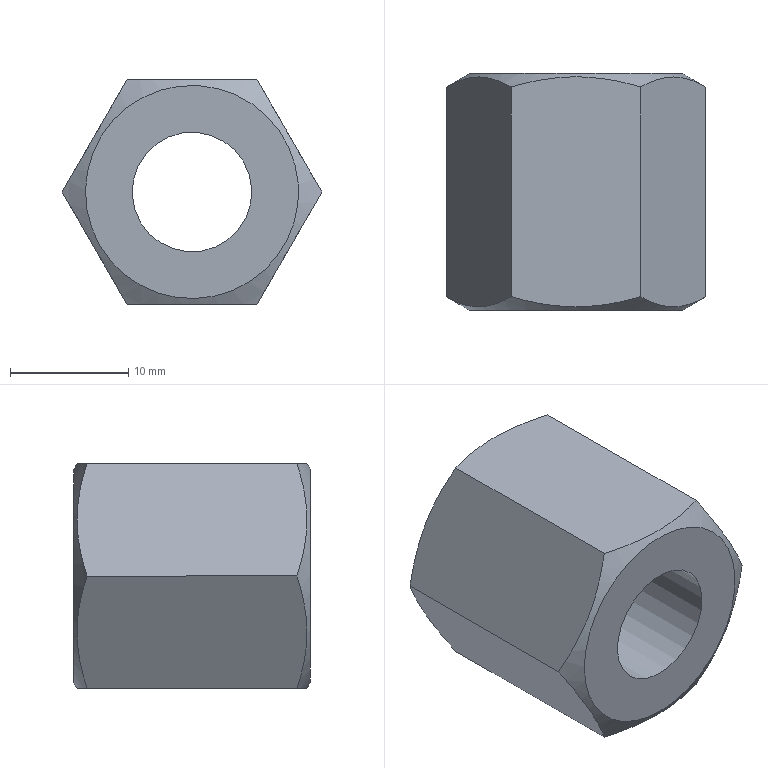Part | NX | features 5003_347_NTFL12-20 2 | 1 solid | 11 faces | box 21.939 x 20 x 19 mm | volume 4608 mm3 | plane 8 | cone 2 | cylinder 1 | commonest cylinder face diameters 10.106 x1
STEP:
#1=CARTESIAN_POINT('',(117.149,13.9,-124.526));
#2=VERTEX_POINT('',#1);
#3=CARTESIAN_POINT('',(121.525,13.9,-122.));
#4=DIRECTION('',(0.,1.,0.));
#5=DIRECTION('',(-0.866,0.,-0.5));
#6=AXIS2_PLACEMENT_3D('',#3,#4,#5);
#7=CIRCLE('',#6,5.053);
#8=EDGE_CURVE('',#2,#2,#7,.F.);
#9=ORIENTED_EDGE('',*,*,#8,.F.);
#10=EDGE_LOOP('',(#9));
#11=FACE_BOUND('',#10,.T.);
#12=CARTESIAN_POINT('',(117.149,-6.1,-124.526));
#13=VERTEX_POINT('',#12);
#14=CARTESIAN_POINT('',(121.525,-6.1,-122.));
#15=DIRECTION('',(0.,1.,0.));
#16=DIRECTION('',(-0.866,0.,-0.5));
#17=AXIS2_PLACEMENT_3D('',#14,#15,#16);
#18=CIRCLE('',#17,5.053);
#19=EDGE_CURVE('',#13,#13,#18,.T.);
#20=ORIENTED_EDGE('',*,*,#19,.F.);
#21=EDGE_LOOP('',(#20));
#22=FACE_BOUND('',#21,.T.);
#23=CARTESIAN_POINT('',(121.525,13.9,-122.));
#24=DIRECTION('',(0.,1.,0.));
#25=DIRECTION('',(-0.866,0.,-0.5));
#26=AXIS2_PLACEMENT_3D('',#23,#24,#25);
#27=CYLINDRICAL_SURFACE('',#26,5.053);
#28=ADVANCED_FACE('',(#11,#22),#27,.F.);
#29=CARTESIAN_POINT('',(113.731,-6.1,-126.5));
#30=VERTEX_POINT('',#29);
#31=CARTESIAN_POINT('',(121.525,-6.1,-122.));
#32=DIRECTION('',(0.,1.,0.));
#33=DIRECTION('',(-0.866,0.,-0.5));
#34=AXIS2_PLACEMENT_3D('',#31,#32,#33);
#35=CIRCLE('',#34,9.);
#36=EDGE_CURVE('',#30,#30,#35,.T.);
#37=ORIENTED_EDGE('',*,*,#36,.F.);
#38=EDGE_LOOP('',(#37));
#39=FACE_BOUND('',#38,.T.);
#40=ORIENTED_EDGE('',*,*,#19,.T.);
#41=EDGE_LOOP('',(#40));
#42=FACE_BOUND('',#41,.T.);
#43=CARTESIAN_POINT('',(121.525,-6.1,-122.));
#44=DIRECTION('',(0.,1.,0.));
#45=DIRECTION('',(-0.866,0.,-0.5));
#46=AXIS2_PLACEMENT_3D('',#43,#44,#45);
#47=PLANE('',#46);
#48=ADVANCED_FACE('',(#39,#42),#47,.F.);
#49=CARTESIAN_POINT('',(129.319,13.9,-117.5));
#50=VERTEX_POINT('',#49);
#51=CARTESIAN_POINT('',(121.525,13.9,-122.));
#52=DIRECTION('',(0.,-1.,0.));
#53=DIRECTION('',(0.866,0.,0.5));
#54=AXIS2_PLACEMENT_3D('',#51,#52,#53);
#55=CIRCLE('',#54,9.);
#56=EDGE_CURVE('',#50,#50,#55,.F.);
#57=ORIENTED_EDGE('',*,*,#56,.T.);
#58=EDGE_LOOP('',(#57));
#59=FACE_BOUND('',#58,.T.);
#60=ORIENTED_EDGE('',*,*,#8,.T.);
#61=EDGE_LOOP('',(#60));
#62=FACE_BOUND('',#61,.T.);
#63=CARTESIAN_POINT('',(121.525,13.9,-122.));
#64=DIRECTION('',(0.,1.,0.));
#65=DIRECTION('',(-0.866,0.,-0.5));
#66=AXIS2_PLACEMENT_3D('',#63,#64,#65);
#67=PLANE('',#66);
#68=ADVANCED_FACE('',(#59,#62),#67,.T.);
#69=ORIENTED_EDGE('',*,*,#36,.T.);
#70=EDGE_LOOP('',(#69));
#71=FACE_BOUND('',#70,.T.);
#72=CARTESIAN_POINT('',(127.01,-4.963,-131.5));
#73=VERTEX_POINT('',#72);
#74=CARTESIAN_POINT('',(132.495,-4.963,-122.));
#75=VERTEX_POINT('',#74);
#76=CARTESIAN_POINT('',(127.01,-4.963,-131.5));
#77=CARTESIAN_POINT('',(127.905,-5.48,-129.949));
#78=CARTESIAN_POINT('',(129.742,-6.142,-126.767));
#79=CARTESIAN_POINT('',(131.598,-5.481,-123.553));
#80=CARTESIAN_POINT('',(132.495,-4.963,-122.));
#81=B_SPLINE_CURVE_WITH_KNOTS('',3,(#76,#77,#78,#79,#80),.UNSPECIFIED.,.F.,.F.,(4,1,4),(0.,0.005539,0.01108),.UNSPECIFIED.);
#82=EDGE_CURVE('',#73,#75,#81,.T.);
#83=ORIENTED_EDGE('',*,*,#82,.T.);
#84=CARTESIAN_POINT('',(127.01,-4.963,-112.5));
#85=VERTEX_POINT('',#84);
#86=CARTESIAN_POINT('',(132.495,-4.963,-122.));
#87=CARTESIAN_POINT('',(131.599,-5.48,-120.448));
#88=CARTESIAN_POINT('',(129.752,-6.143,-117.25));
#89=CARTESIAN_POINT('',(127.906,-5.48,-114.052));
#90=CARTESIAN_POINT('',(127.01,-4.963,-112.5));
#91=B_SPLINE_CURVE_WITH_KNOTS('',3,(#86,#87,#88,#89,#90),.UNSPECIFIED.,.F.,.F.,(4,1,4),(0.,0.00555,0.0111),.UNSPECIFIED.);
#92=EDGE_CURVE('',#75,#85,#91,.T.);
#93=ORIENTED_EDGE('',*,*,#92,.T.);
#94=CARTESIAN_POINT('',(116.04,-4.963,-112.5));
#95=VERTEX_POINT('',#94);
#96=CARTESIAN_POINT('',(127.01,-4.963,-112.5));
#97=CARTESIAN_POINT('',(125.219,-5.48,-112.5));
#98=CARTESIAN_POINT('',(121.545,-6.142,-112.5));
#99=CARTESIAN_POINT('',(117.834,-5.481,-112.5));
#100=CARTESIAN_POINT('',(116.04,-4.963,-112.5));
#101=B_SPLINE_CURVE_WITH_KNOTS('',3,(#96,#97,#98,#99,#100),.UNSPECIFIED.,.F.,.F.,(4,1,4),(0.,0.005539,0.01108),.UNSPECIFIED.);
#102=EDGE_CURVE('',#85,#95,#101,.T.);
#103=ORIENTED_EDGE('',*,*,#102,.T.);
#104=CARTESIAN_POINT('',(110.555,-4.963,-122.));
#105=VERTEX_POINT('',#104);
#106=CARTESIAN_POINT('',(116.04,-4.963,-112.5));
#107=CARTESIAN_POINT('',(115.145,-5.48,-114.051));
#108=CARTESIAN_POINT('',(113.308,-6.142,-117.233));
#109=CARTESIAN_POINT('',(111.452,-5.481,-120.447));
#110=CARTESIAN_POINT('',(110.555,-4.963,-122.));
#111=B_SPLINE_CURVE_WITH_KNOTS('',3,(#106,#107,#108,#109,#110),.UNSPECIFIED.,.F.,.F.,(4,1,4),(0.,0.005539,0.01108),.UNSPECIFIED.);
#112=EDGE_CURVE('',#95,#105,#111,.T.);
#113=ORIENTED_EDGE('',*,*,#112,.T.);
#114=CARTESIAN_POINT('',(116.04,-4.963,-131.5));
#115=VERTEX_POINT('',#114);
#116=CARTESIAN_POINT('',(110.555,-4.963,-122.));
#117=CARTESIAN_POINT('',(111.451,-5.48,-123.552));
#118=CARTESIAN_POINT('',(113.298,-6.143,-126.75));
#119=CARTESIAN_POINT('',(115.144,-5.48,-129.948));
#120=CARTESIAN_POINT('',(116.04,-4.963,-131.5));
#121=B_SPLINE_CURVE_WITH_KNOTS('',3,(#116,#117,#118,#119,#120),.UNSPECIFIED.,.F.,.F.,(4,1,4),(-0.00555,0.,0.00555),.UNSPECIFIED.);
#122=EDGE_CURVE('',#105,#115,#121,.T.);
#123=ORIENTED_EDGE('',*,*,#122,.T.);
#124=CARTESIAN_POINT('',(116.04,-4.963,-131.5));
#125=CARTESIAN_POINT('',(117.831,-5.48,-131.5));
#126=CARTESIAN_POINT('',(121.505,-6.142,-131.5));
#127=CARTESIAN_POINT('',(125.216,-5.481,-131.5));
#128=CARTESIAN_POINT('',(127.01,-4.963,-131.5));
#129=B_SPLINE_CURVE_WITH_KNOTS('',3,(#124,#125,#126,#127,#128),.UNSPECIFIED.,.F.,.F.,(4,1,4),(0.,0.005539,0.01108),.UNSPECIFIED.);
#130=EDGE_CURVE('',#115,#73,#129,.T.);
#131=ORIENTED_EDGE('',*,*,#130,.T.);
#132=EDGE_LOOP('',(#83,#93,#103,#113,#123,#131));
#133=FACE_BOUND('',#132,.T.);
#134=CARTESIAN_POINT('',(121.525,-4.956,-122.));
#135=DIRECTION('',(0.,1.,0.));
#136=DIRECTION('',(-0.866,0.,-0.5));
#137=AXIS2_PLACEMENT_3D('',#134,#135,#136);
#138=CONICAL_SURFACE('',#137,10.981,1.047);
#139=ADVANCED_FACE('',(#71,#133),#138,.T.);
#140=ORIENTED_EDGE('',*,*,#56,.F.);
#141=EDGE_LOOP('',(#140));
#142=FACE_BOUND('',#141,.T.);
#143=CARTESIAN_POINT('',(127.01,12.763,-131.5));
#144=VERTEX_POINT('',#143);
#145=CARTESIAN_POINT('',(116.04,12.763,-131.5));
#146=VERTEX_POINT('',#145);
#147=CARTESIAN_POINT('',(127.01,12.763,-131.5));
#148=CARTESIAN_POINT('',(125.219,13.28,-131.5));
#149=CARTESIAN_POINT('',(121.545,13.942,-131.5));
#150=CARTESIAN_POINT('',(117.834,13.281,-131.5));
#151=CARTESIAN_POINT('',(116.04,12.763,-131.5));
#152=B_SPLINE_CURVE_WITH_KNOTS('',3,(#147,#148,#149,#150,#151),.UNSPECIFIED.,.F.,.F.,(4,1,4),(0.,0.005539,0.01108),.UNSPECIFIED.);
#153=EDGE_CURVE('',#144,#146,#152,.T.);
#154=ORIENTED_EDGE('',*,*,#153,.T.);
#155=CARTESIAN_POINT('',(110.555,12.763,-122.));
#156=VERTEX_POINT('',#155);
#157=CARTESIAN_POINT('',(116.04,12.763,-131.5));
#158=CARTESIAN_POINT('',(115.144,13.28,-129.948));
#159=CARTESIAN_POINT('',(113.298,13.943,-126.75));
#160=CARTESIAN_POINT('',(111.451,13.28,-123.552));
#161=CARTESIAN_POINT('',(110.555,12.763,-122.));
#162=B_SPLINE_CURVE_WITH_KNOTS('',3,(#157,#158,#159,#160,#161),.UNSPECIFIED.,.F.,.F.,(4,1,4),(0.,0.00555,0.0111),.UNSPECIFIED.);
#163=EDGE_CURVE('',#146,#156,#162,.T.);
#164=ORIENTED_EDGE('',*,*,#163,.T.);
#165=CARTESIAN_POINT('',(116.04,12.763,-112.5));
#166=VERTEX_POINT('',#165);
#167=CARTESIAN_POINT('',(110.555,12.763,-122.));
#168=CARTESIAN_POINT('',(111.451,13.28,-120.449));
#169=CARTESIAN_POINT('',(113.288,13.942,-117.267));
#170=CARTESIAN_POINT('',(115.143,13.281,-114.053));
#171=CARTESIAN_POINT('',(116.04,12.763,-112.5));
#172=B_SPLINE_CURVE_WITH_KNOTS('',3,(#167,#168,#169,#170,#171),.UNSPECIFIED.,.F.,.F.,(4,1,4),(0.,0.005539,0.01108),.UNSPECIFIED.);
#173=EDGE_CURVE('',#156,#166,#172,.T.);
#174=ORIENTED_EDGE('',*,*,#173,.T.);
#175=CARTESIAN_POINT('',(127.01,12.763,-112.5));
#176=VERTEX_POINT('',#175);
#177=CARTESIAN_POINT('',(116.04,12.763,-112.5));
#178=CARTESIAN_POINT('',(117.831,13.28,-112.5));
#179=CARTESIAN_POINT('',(121.505,13.942,-112.5));
#180=CARTESIAN_POINT('',(125.216,13.281,-112.5));
#181=CARTESIAN_POINT('',(127.01,12.763,-112.5));
#182=B_SPLINE_CURVE_WITH_KNOTS('',3,(#177,#178,#179,#180,#181),.UNSPECIFIED.,.F.,.F.,(4,1,4),(0.,0.005539,0.01108),.UNSPECIFIED.);
#183=EDGE_CURVE('',#166,#176,#182,.T.);
#184=ORIENTED_EDGE('',*,*,#183,.T.);
#185=CARTESIAN_POINT('',(132.495,12.763,-122.));
#186=VERTEX_POINT('',#185);
#187=CARTESIAN_POINT('',(127.01,12.763,-112.5));
#188=CARTESIAN_POINT('',(127.906,13.28,-114.052));
#189=CARTESIAN_POINT('',(129.752,13.943,-117.25));
#190=CARTESIAN_POINT('',(131.599,13.28,-120.448));
#191=CARTESIAN_POINT('',(132.495,12.763,-122.));
#192=B_SPLINE_CURVE_WITH_KNOTS('',3,(#187,#188,#189,#190,#191),.UNSPECIFIED.,.F.,.F.,(4,1,4),(-0.00555,0.,0.00555),.UNSPECIFIED.);
#193=EDGE_CURVE('',#176,#186,#192,.T.);
#194=ORIENTED_EDGE('',*,*,#193,.T.);
#195=CARTESIAN_POINT('',(132.495,12.763,-122.));
#196=CARTESIAN_POINT('',(131.599,13.28,-123.551));
#197=CARTESIAN_POINT('',(129.762,13.942,-126.733));
#198=CARTESIAN_POINT('',(127.907,13.281,-129.947));
#199=CARTESIAN_POINT('',(127.01,12.763,-131.5));
#200=B_SPLINE_CURVE_WITH_KNOTS('',3,(#195,#196,#197,#198,#199),.UNSPECIFIED.,.F.,.F.,(4,1,4),(0.,0.005539,0.01108),.UNSPECIFIED.);
#201=EDGE_CURVE('',#186,#144,#200,.T.);
#202=ORIENTED_EDGE('',*,*,#201,.T.);
#203=EDGE_LOOP('',(#154,#164,#174,#184,#194,#202));
#204=FACE_BOUND('',#203,.T.);
#205=CARTESIAN_POINT('',(121.525,12.756,-122.));
#206=DIRECTION('',(0.,-1.,0.));
#207=DIRECTION('',(0.866,0.,0.5));
#208=AXIS2_PLACEMENT_3D('',#205,#206,#207);
#209=CONICAL_SURFACE('',#208,10.981,1.047);
#210=ADVANCED_FACE('',(#142,#204),#209,.T.);
#211=CARTESIAN_POINT('',(127.01,-6.1,-112.5));
#212=DIRECTION('',(0.,1.,0.));
#213=VECTOR('',#212,1000.);
#214=LINE('',#211,#213);
#215=EDGE_CURVE('',#176,#85,#214,.F.);
#216=ORIENTED_EDGE('',*,*,#215,.T.);
#217=ORIENTED_EDGE('',*,*,#92,.F.);
#218=CARTESIAN_POINT('',(132.495,-6.1,-122.));
#219=DIRECTION('',(0.,1.,0.));
#220=VECTOR('',#219,1000.);
#221=LINE('',#218,#220);
#222=EDGE_CURVE('',#75,#186,#221,.T.);
#223=ORIENTED_EDGE('',*,*,#222,.T.);
#224=ORIENTED_EDGE('',*,*,#193,.F.);
#225=EDGE_LOOP('',(#216,#217,#223,#224));
#226=FACE_BOUND('',#225,.T.);
#227=CARTESIAN_POINT('',(127.01,-6.1,-112.5));
#228=DIRECTION('',(0.866,0.,0.5));
#229=DIRECTION('',(0.,1.,0.));
#230=AXIS2_PLACEMENT_3D('',#227,#228,#229);
#231=PLANE('',#230);
#232=ADVANCED_FACE('',(#226),#231,.T.);
#233=ORIENTED_EDGE('',*,*,#222,.F.);
#234=ORIENTED_EDGE('',*,*,#82,.F.);
#235=CARTESIAN_POINT('',(127.01,-6.1,-131.5));
#236=DIRECTION('',(0.,1.,0.));
#237=VECTOR('',#236,1000.);
#238=LINE('',#235,#237);
#239=EDGE_CURVE('',#73,#144,#238,.T.);
#240=ORIENTED_EDGE('',*,*,#239,.T.);
#241=ORIENTED_EDGE('',*,*,#201,.F.);
#242=EDGE_LOOP('',(#233,#234,#240,#241));
#243=FACE_BOUND('',#242,.T.);
#244=CARTESIAN_POINT('',(132.495,-6.1,-122.));
#245=DIRECTION('',(0.866,0.,-0.5));
#246=DIRECTION('',(-0.5,0.,-0.866));
#247=AXIS2_PLACEMENT_3D('',#244,#245,#246);
#248=PLANE('',#247);
#249=ADVANCED_FACE('',(#243),#248,.T.);
#250=ORIENTED_EDGE('',*,*,#239,.F.);
#251=ORIENTED_EDGE('',*,*,#130,.F.);
#252=CARTESIAN_POINT('',(116.04,-6.1,-131.5));
#253=DIRECTION('',(0.,1.,0.));
#254=VECTOR('',#253,1000.);
#255=LINE('',#252,#254);
#256=EDGE_CURVE('',#115,#146,#255,.T.);
#257=ORIENTED_EDGE('',*,*,#256,.T.);
#258=ORIENTED_EDGE('',*,*,#153,.F.);
#259=EDGE_LOOP('',(#250,#251,#257,#258));
#260=FACE_BOUND('',#259,.T.);
#261=CARTESIAN_POINT('',(127.01,-6.1,-131.5));
#262=DIRECTION('',(0.,0.,-1.));
#263=DIRECTION('',(-1.,0.,0.));
#264=AXIS2_PLACEMENT_3D('',#261,#262,#263);
#265=PLANE('',#264);
#266=ADVANCED_FACE('',(#260),#265,.T.);
#267=ORIENTED_EDGE('',*,*,#122,.F.);
#268=CARTESIAN_POINT('',(110.555,-6.1,-122.));
#269=DIRECTION('',(0.,-1.,0.));
#270=VECTOR('',#269,1000.);
#271=LINE('',#268,#270);
#272=EDGE_CURVE('',#105,#156,#271,.F.);
#273=ORIENTED_EDGE('',*,*,#272,.T.);
#274=ORIENTED_EDGE('',*,*,#163,.F.);
#275=ORIENTED_EDGE('',*,*,#256,.F.);
#276=EDGE_LOOP('',(#267,#273,#274,#275));
#277=FACE_BOUND('',#276,.T.);
#278=CARTESIAN_POINT('',(116.04,-6.1,-131.5));
#279=DIRECTION('',(-0.866,0.,-0.5));
#280=DIRECTION('',(0.,-1.,0.));
#281=AXIS2_PLACEMENT_3D('',#278,#279,#280);
#282=PLANE('',#281);
#283=ADVANCED_FACE('',(#277),#282,.T.);
#284=ORIENTED_EDGE('',*,*,#272,.F.);
#285=ORIENTED_EDGE('',*,*,#112,.F.);
#286=CARTESIAN_POINT('',(116.04,-6.1,-112.5));
#287=DIRECTION('',(0.,1.,0.));
#288=VECTOR('',#287,1000.);
#289=LINE('',#286,#288);
#290=EDGE_CURVE('',#95,#166,#289,.T.);
#291=ORIENTED_EDGE('',*,*,#290,.T.);
#292=ORIENTED_EDGE('',*,*,#173,.F.);
#293=EDGE_LOOP('',(#284,#285,#291,#292));
#294=FACE_BOUND('',#293,.T.);
#295=CARTESIAN_POINT('',(110.555,-6.1,-122.));
#296=DIRECTION('',(-0.866,0.,0.5));
#297=DIRECTION('',(0.5,0.,0.866));
#298=AXIS2_PLACEMENT_3D('',#295,#296,#297);
#299=PLANE('',#298);
#300=ADVANCED_FACE('',(#294),#299,.T.);
#301=ORIENTED_EDGE('',*,*,#290,.F.);
#302=ORIENTED_EDGE('',*,*,#102,.F.);
#303=ORIENTED_EDGE('',*,*,#215,.F.);
#304=ORIENTED_EDGE('',*,*,#183,.F.);
#305=EDGE_LOOP('',(#301,#302,#303,#304));
#306=FACE_BOUND('',#305,.T.);
#307=CARTESIAN_POINT('',(116.04,-6.1,-112.5));
#308=DIRECTION('',(0.,0.,1.));
#309=DIRECTION('',(1.,0.,0.));
#310=AXIS2_PLACEMENT_3D('',#307,#308,#309);
#311=PLANE('',#310);
#312=ADVANCED_FACE('',(#306),#311,.T.);
#313=CLOSED_SHELL('',(#28,#48,#68,#139,#210,#232,#249,#266,#283,#300,#312));
#314=MANIFOLD_SOLID_BREP('',#313);
#315=(LENGTH_UNIT()NAMED_UNIT(*)SI_UNIT(.MILLI.,.METRE.));
#316=UNCERTAINTY_MEASURE_WITH_UNIT(LENGTH_MEASURE(0.0508),#315,'','');
#317=(NAMED_UNIT(*)PLANE_ANGLE_UNIT()SI_UNIT($,.RADIAN.));
#318=(NAMED_UNIT(*)SI_UNIT($,.STERADIAN.)SOLID_ANGLE_UNIT());
#319=(GEOMETRIC_REPRESENTATION_CONTEXT(3)GLOBAL_UNCERTAINTY_ASSIGNED_CONTEXT((#316))GLOBAL_UNIT_ASSIGNED_CONTEXT((#315,#317,#318))REPRESENTATION_CONTEXT('',''));
#320=ADVANCED_BREP_SHAPE_REPRESENTATION('',(#314),#319);